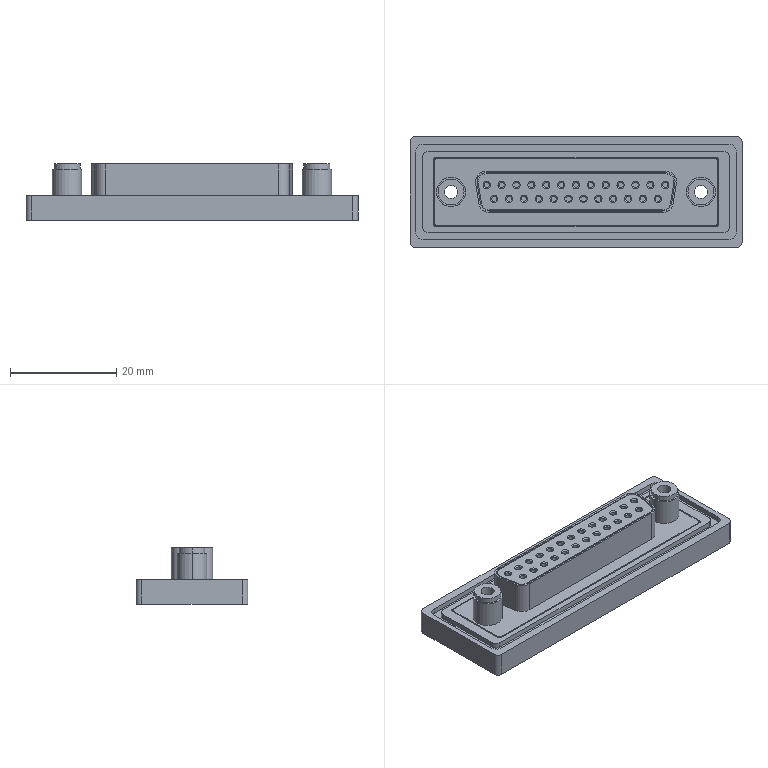Part | SolidWorks | features BaseBody 1 | 1 solid | 217 faces | box 62.5 x 21 x 10.6 mm | volume 7477 mm3 | cylinder 97 | plane 70 | cone 50 | commonest cylinder face diameters 1 x58 3 x9 2 x8 3.4 x5 4 x5 2.5 x4